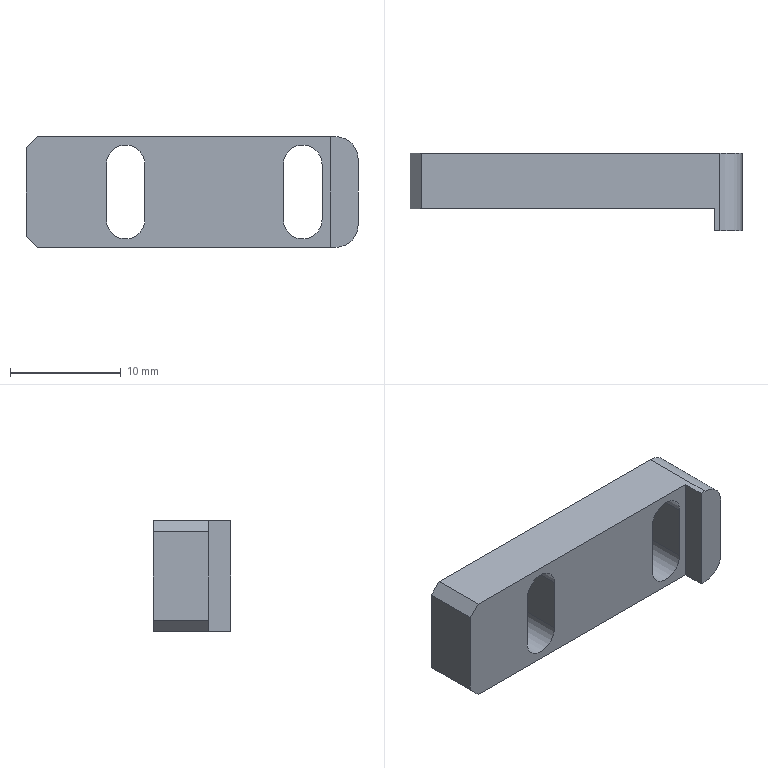Part | SolidWorks | features Chamfer 1, Extrusion 1, Fillet 1, ICE 1 | 1 solid | 20 faces | box 30 x 7 x 10 mm | volume 1262 mm3 | plane 14 | cylinder 6 | commonest cylinder face diameters 3.5 x4 4 x2
STEP:
#1=CARTESIAN_POINT('',(0.,-7.,3.));
#2=VERTEX_POINT('',#1);
#3=CARTESIAN_POINT('',(0.,-7.,-3.));
#4=VERTEX_POINT('',#3);
#5=CARTESIAN_POINT('',(0.,-7.,5.));
#6=DIRECTION('',(0.,0.,-1.));
#7=VECTOR('',#6,1000.);
#8=LINE('',#5,#7);
#9=EDGE_CURVE('',#2,#4,#8,.T.);
#10=ORIENTED_EDGE('',*,*,#9,.T.);
#11=CARTESIAN_POINT('',(0.,0.,-3.));
#12=VERTEX_POINT('',#11);
#13=CARTESIAN_POINT('',(0.,0.,-3.));
#14=DIRECTION('',(0.,1.,0.));
#15=VECTOR('',#14,1000.);
#16=LINE('',#13,#15);
#17=EDGE_CURVE('',#4,#12,#16,.T.);
#18=ORIENTED_EDGE('',*,*,#17,.T.);
#19=CARTESIAN_POINT('',(0.,0.,3.));
#20=VERTEX_POINT('',#19);
#21=CARTESIAN_POINT('',(0.,0.,5.));
#22=DIRECTION('',(0.,0.,-1.));
#23=VECTOR('',#22,1000.);
#24=LINE('',#21,#23);
#25=EDGE_CURVE('',#20,#12,#24,.T.);
#26=ORIENTED_EDGE('',*,*,#25,.F.);
#27=CARTESIAN_POINT('',(0.,0.,3.));
#28=DIRECTION('',(0.,-1.,0.));
#29=VECTOR('',#28,1000.);
#30=LINE('',#27,#29);
#31=EDGE_CURVE('',#20,#2,#30,.T.);
#32=ORIENTED_EDGE('',*,*,#31,.T.);
#33=EDGE_LOOP('',(#10,#18,#26,#32));
#34=FACE_OUTER_BOUND('',#33,.T.);
#35=CARTESIAN_POINT('',(0.,0.,5.));
#36=DIRECTION('',(-1.,0.,0.));
#37=DIRECTION('',(0.,-1.,0.));
#38=AXIS2_PLACEMENT_3D('',#35,#36,#37);
#39=PLANE('',#38);
#40=ADVANCED_FACE('',(#34),#39,.F.);
#41=CARTESIAN_POINT('',(-3.25,0.,-2.5));
#42=VERTEX_POINT('',#41);
#43=CARTESIAN_POINT('',(-3.25,0.,2.5));
#44=VERTEX_POINT('',#43);
#45=CARTESIAN_POINT('',(-3.25,0.,2.5));
#46=DIRECTION('',(0.,0.,1.));
#47=VECTOR('',#46,1000.);
#48=LINE('',#45,#47);
#49=EDGE_CURVE('',#42,#44,#48,.T.);
#50=ORIENTED_EDGE('',*,*,#49,.T.);
#51=CARTESIAN_POINT('',(-6.75,0.,2.5));
#52=VERTEX_POINT('',#51);
#53=CARTESIAN_POINT('',(-5.,0.,2.5));
#54=DIRECTION('',(0.,-1.,0.));
#55=DIRECTION('',(1.,0.,0.));
#56=AXIS2_PLACEMENT_3D('',#53,#54,#55);
#57=CIRCLE('',#56,1.75);
#58=EDGE_CURVE('',#44,#52,#57,.T.);
#59=ORIENTED_EDGE('',*,*,#58,.T.);
#60=CARTESIAN_POINT('',(-6.75,0.,-2.5));
#61=VERTEX_POINT('',#60);
#62=CARTESIAN_POINT('',(-6.75,0.,2.5));
#63=DIRECTION('',(0.,0.,-1.));
#64=VECTOR('',#63,1000.);
#65=LINE('',#62,#64);
#66=EDGE_CURVE('',#52,#61,#65,.T.);
#67=ORIENTED_EDGE('',*,*,#66,.T.);
#68=CARTESIAN_POINT('',(-5.,0.,-2.5));
#69=DIRECTION('',(0.,-1.,0.));
#70=DIRECTION('',(1.,0.,0.));
#71=AXIS2_PLACEMENT_3D('',#68,#69,#70);
#72=CIRCLE('',#71,1.75);
#73=EDGE_CURVE('',#61,#42,#72,.T.);
#74=ORIENTED_EDGE('',*,*,#73,.T.);
#75=EDGE_LOOP('',(#50,#59,#67,#74));
#76=FACE_BOUND('',#75,.T.);
#77=CARTESIAN_POINT('',(-19.25,0.,-2.5));
#78=VERTEX_POINT('',#77);
#79=CARTESIAN_POINT('',(-19.25,0.,2.5));
#80=VERTEX_POINT('',#79);
#81=CARTESIAN_POINT('',(-19.25,0.,2.5));
#82=DIRECTION('',(0.,0.,1.));
#83=VECTOR('',#82,1000.);
#84=LINE('',#81,#83);
#85=EDGE_CURVE('',#78,#80,#84,.T.);
#86=ORIENTED_EDGE('',*,*,#85,.T.);
#87=CARTESIAN_POINT('',(-22.75,0.,2.5));
#88=VERTEX_POINT('',#87);
#89=CARTESIAN_POINT('',(-21.,0.,2.5));
#90=DIRECTION('',(0.,-1.,0.));
#91=DIRECTION('',(1.,0.,0.));
#92=AXIS2_PLACEMENT_3D('',#89,#90,#91);
#93=CIRCLE('',#92,1.75);
#94=EDGE_CURVE('',#80,#88,#93,.T.);
#95=ORIENTED_EDGE('',*,*,#94,.T.);
#96=CARTESIAN_POINT('',(-22.75,0.,-2.5));
#97=VERTEX_POINT('',#96);
#98=CARTESIAN_POINT('',(-22.75,0.,2.5));
#99=DIRECTION('',(0.,0.,-1.));
#100=VECTOR('',#99,1000.);
#101=LINE('',#98,#100);
#102=EDGE_CURVE('',#88,#97,#101,.T.);
#103=ORIENTED_EDGE('',*,*,#102,.T.);
#104=CARTESIAN_POINT('',(-21.,0.,-2.5));
#105=DIRECTION('',(0.,-1.,0.));
#106=DIRECTION('',(1.,0.,0.));
#107=AXIS2_PLACEMENT_3D('',#104,#105,#106);
#108=CIRCLE('',#107,1.75);
#109=EDGE_CURVE('',#97,#78,#108,.T.);
#110=ORIENTED_EDGE('',*,*,#109,.T.);
#111=EDGE_LOOP('',(#86,#95,#103,#110));
#112=FACE_BOUND('',#111,.T.);
#113=CARTESIAN_POINT('',(-30.,0.,4.));
#114=VERTEX_POINT('',#113);
#115=CARTESIAN_POINT('',(-30.,0.,-4.));
#116=VERTEX_POINT('',#115);
#117=CARTESIAN_POINT('',(-30.,0.,5.));
#118=DIRECTION('',(0.,0.,-1.));
#119=VECTOR('',#118,1000.);
#120=LINE('',#117,#119);
#121=EDGE_CURVE('',#114,#116,#120,.T.);
#122=ORIENTED_EDGE('',*,*,#121,.F.);
#123=CARTESIAN_POINT('',(-29.,0.,5.));
#124=VERTEX_POINT('',#123);
#125=CARTESIAN_POINT('',(-29.,0.,5.));
#126=DIRECTION('',(0.7071,0.,0.7071));
#127=VECTOR('',#126,1000.);
#128=LINE('',#125,#127);
#129=EDGE_CURVE('',#114,#124,#128,.T.);
#130=ORIENTED_EDGE('',*,*,#129,.T.);
#131=CARTESIAN_POINT('',(-2.,0.,5.));
#132=VERTEX_POINT('',#131);
#133=CARTESIAN_POINT('',(0.,0.,5.));
#134=DIRECTION('',(-1.,0.,0.));
#135=VECTOR('',#134,1000.);
#136=LINE('',#133,#135);
#137=EDGE_CURVE('',#132,#124,#136,.T.);
#138=ORIENTED_EDGE('',*,*,#137,.F.);
#139=CARTESIAN_POINT('',(-2.,0.,3.));
#140=DIRECTION('',(0.,1.,0.));
#141=DIRECTION('',(1.,0.,0.));
#142=AXIS2_PLACEMENT_3D('',#139,#140,#141);
#143=CIRCLE('',#142,2.);
#144=EDGE_CURVE('',#132,#20,#143,.T.);
#145=ORIENTED_EDGE('',*,*,#144,.T.);
#146=ORIENTED_EDGE('',*,*,#25,.T.);
#147=CARTESIAN_POINT('',(-2.,0.,-5.));
#148=VERTEX_POINT('',#147);
#149=CARTESIAN_POINT('',(-2.,0.,-3.));
#150=DIRECTION('',(0.,1.,0.));
#151=DIRECTION('',(1.,0.,0.));
#152=AXIS2_PLACEMENT_3D('',#149,#150,#151);
#153=CIRCLE('',#152,2.);
#154=EDGE_CURVE('',#12,#148,#153,.T.);
#155=ORIENTED_EDGE('',*,*,#154,.T.);
#156=CARTESIAN_POINT('',(-29.,0.,-5.));
#157=VERTEX_POINT('',#156);
#158=CARTESIAN_POINT('',(0.,0.,-5.));
#159=DIRECTION('',(-1.,0.,0.));
#160=VECTOR('',#159,1000.);
#161=LINE('',#158,#160);
#162=EDGE_CURVE('',#148,#157,#161,.T.);
#163=ORIENTED_EDGE('',*,*,#162,.T.);
#164=CARTESIAN_POINT('',(-30.,0.,-4.));
#165=DIRECTION('',(-0.7071,0.,0.7071));
#166=VECTOR('',#165,1000.);
#167=LINE('',#164,#166);
#168=EDGE_CURVE('',#157,#116,#167,.T.);
#169=ORIENTED_EDGE('',*,*,#168,.T.);
#170=EDGE_LOOP('',(#122,#130,#138,#145,#146,#155,#163,#169));
#171=FACE_OUTER_BOUND('',#170,.T.);
#172=CARTESIAN_POINT('',(0.,0.,5.));
#173=DIRECTION('',(0.,-1.,0.));
#174=DIRECTION('',(1.,0.,0.));
#175=AXIS2_PLACEMENT_3D('',#172,#173,#174);
#176=PLANE('',#175);
#177=ADVANCED_FACE('',(#76,#112,#171),#176,.F.);
#178=CARTESIAN_POINT('',(-30.,-5.,4.));
#179=VERTEX_POINT('',#178);
#180=CARTESIAN_POINT('',(-30.,-5.,-4.));
#181=VERTEX_POINT('',#180);
#182=CARTESIAN_POINT('',(-30.,-5.,5.));
#183=DIRECTION('',(0.,0.,-1.));
#184=VECTOR('',#183,1000.);
#185=LINE('',#182,#184);
#186=EDGE_CURVE('',#179,#181,#185,.T.);
#187=ORIENTED_EDGE('',*,*,#186,.F.);
#188=CARTESIAN_POINT('',(-30.,0.,4.));
#189=DIRECTION('',(0.,1.,0.));
#190=VECTOR('',#189,1000.);
#191=LINE('',#188,#190);
#192=EDGE_CURVE('',#179,#114,#191,.T.);
#193=ORIENTED_EDGE('',*,*,#192,.T.);
#194=ORIENTED_EDGE('',*,*,#121,.T.);
#195=CARTESIAN_POINT('',(-30.,-5.,-4.));
#196=DIRECTION('',(0.,-1.,0.));
#197=VECTOR('',#196,1000.);
#198=LINE('',#195,#197);
#199=EDGE_CURVE('',#116,#181,#198,.T.);
#200=ORIENTED_EDGE('',*,*,#199,.T.);
#201=EDGE_LOOP('',(#187,#193,#194,#200));
#202=FACE_OUTER_BOUND('',#201,.T.);
#203=CARTESIAN_POINT('',(-30.,0.,5.));
#204=DIRECTION('',(1.,0.,0.));
#205=DIRECTION('',(0.,0.,-1.));
#206=AXIS2_PLACEMENT_3D('',#203,#204,#205);
#207=PLANE('',#206);
#208=ADVANCED_FACE('',(#202),#207,.F.);
#209=CARTESIAN_POINT('',(-6.75,-5.,2.5));
#210=VERTEX_POINT('',#209);
#211=CARTESIAN_POINT('',(-6.75,-5.,-2.5));
#212=VERTEX_POINT('',#211);
#213=CARTESIAN_POINT('',(-6.75,-5.,2.5));
#214=DIRECTION('',(0.,0.,-1.));
#215=VECTOR('',#214,1000.);
#216=LINE('',#213,#215);
#217=EDGE_CURVE('',#210,#212,#216,.T.);
#218=ORIENTED_EDGE('',*,*,#217,.F.);
#219=CARTESIAN_POINT('',(-3.25,-5.,2.5));
#220=VERTEX_POINT('',#219);
#221=CARTESIAN_POINT('',(-5.,-5.,2.5));
#222=DIRECTION('',(0.,-1.,0.));
#223=DIRECTION('',(1.,0.,0.));
#224=AXIS2_PLACEMENT_3D('',#221,#222,#223);
#225=CIRCLE('',#224,1.75);
#226=EDGE_CURVE('',#220,#210,#225,.T.);
#227=ORIENTED_EDGE('',*,*,#226,.F.);
#228=CARTESIAN_POINT('',(-3.25,-5.,-2.5));
#229=VERTEX_POINT('',#228);
#230=CARTESIAN_POINT('',(-3.25,-5.,2.5));
#231=DIRECTION('',(0.,0.,1.));
#232=VECTOR('',#231,1000.);
#233=LINE('',#230,#232);
#234=EDGE_CURVE('',#229,#220,#233,.T.);
#235=ORIENTED_EDGE('',*,*,#234,.F.);
#236=CARTESIAN_POINT('',(-5.,-5.,-2.5));
#237=DIRECTION('',(0.,-1.,0.));
#238=DIRECTION('',(1.,0.,0.));
#239=AXIS2_PLACEMENT_3D('',#236,#237,#238);
#240=CIRCLE('',#239,1.75);
#241=EDGE_CURVE('',#212,#229,#240,.T.);
#242=ORIENTED_EDGE('',*,*,#241,.F.);
#243=EDGE_LOOP('',(#218,#227,#235,#242));
#244=FACE_BOUND('',#243,.T.);
#245=CARTESIAN_POINT('',(-22.75,-5.,2.5));
#246=VERTEX_POINT('',#245);
#247=CARTESIAN_POINT('',(-22.75,-5.,-2.5));
#248=VERTEX_POINT('',#247);
#249=CARTESIAN_POINT('',(-22.75,-5.,2.5));
#250=DIRECTION('',(0.,0.,-1.));
#251=VECTOR('',#250,1000.);
#252=LINE('',#249,#251);
#253=EDGE_CURVE('',#246,#248,#252,.T.);
#254=ORIENTED_EDGE('',*,*,#253,.F.);
#255=CARTESIAN_POINT('',(-19.25,-5.,2.5));
#256=VERTEX_POINT('',#255);
#257=CARTESIAN_POINT('',(-21.,-5.,2.5));
#258=DIRECTION('',(0.,-1.,0.));
#259=DIRECTION('',(1.,0.,0.));
#260=AXIS2_PLACEMENT_3D('',#257,#258,#259);
#261=CIRCLE('',#260,1.75);
#262=EDGE_CURVE('',#256,#246,#261,.T.);
#263=ORIENTED_EDGE('',*,*,#262,.F.);
#264=CARTESIAN_POINT('',(-19.25,-5.,-2.5));
#265=VERTEX_POINT('',#264);
#266=CARTESIAN_POINT('',(-19.25,-5.,2.5));
#267=DIRECTION('',(0.,0.,1.));
#268=VECTOR('',#267,1000.);
#269=LINE('',#266,#268);
#270=EDGE_CURVE('',#265,#256,#269,.T.);
#271=ORIENTED_EDGE('',*,*,#270,.F.);
#272=CARTESIAN_POINT('',(-21.,-5.,-2.5));
#273=DIRECTION('',(0.,-1.,0.));
#274=DIRECTION('',(1.,0.,0.));
#275=AXIS2_PLACEMENT_3D('',#272,#273,#274);
#276=CIRCLE('',#275,1.75);
#277=EDGE_CURVE('',#248,#265,#276,.T.);
#278=ORIENTED_EDGE('',*,*,#277,.F.);
#279=EDGE_LOOP('',(#254,#263,#271,#278));
#280=FACE_BOUND('',#279,.T.);
#281=CARTESIAN_POINT('',(-29.,-5.,5.));
#282=VERTEX_POINT('',#281);
#283=CARTESIAN_POINT('',(-2.5,-5.,5.));
#284=VERTEX_POINT('',#283);
#285=CARTESIAN_POINT('',(-30.,-5.,5.));
#286=DIRECTION('',(1.,0.,0.));
#287=VECTOR('',#286,1000.);
#288=LINE('',#285,#287);
#289=EDGE_CURVE('',#282,#284,#288,.T.);
#290=ORIENTED_EDGE('',*,*,#289,.F.);
#291=CARTESIAN_POINT('',(-29.,-5.,5.));
#292=DIRECTION('',(-0.7071,0.,-0.7071));
#293=VECTOR('',#292,1000.);
#294=LINE('',#291,#293);
#295=EDGE_CURVE('',#282,#179,#294,.T.);
#296=ORIENTED_EDGE('',*,*,#295,.T.);
#297=ORIENTED_EDGE('',*,*,#186,.T.);
#298=CARTESIAN_POINT('',(-29.,-5.,-5.));
#299=VERTEX_POINT('',#298);
#300=CARTESIAN_POINT('',(-30.,-5.,-4.));
#301=DIRECTION('',(0.7071,0.,-0.7071));
#302=VECTOR('',#301,1000.);
#303=LINE('',#300,#302);
#304=EDGE_CURVE('',#181,#299,#303,.T.);
#305=ORIENTED_EDGE('',*,*,#304,.T.);
#306=CARTESIAN_POINT('',(-2.5,-5.,-5.));
#307=VERTEX_POINT('',#306);
#308=CARTESIAN_POINT('',(-30.,-5.,-5.));
#309=DIRECTION('',(1.,0.,0.));
#310=VECTOR('',#309,1000.);
#311=LINE('',#308,#310);
#312=EDGE_CURVE('',#299,#307,#311,.T.);
#313=ORIENTED_EDGE('',*,*,#312,.T.);
#314=CARTESIAN_POINT('',(-2.5,-5.,5.));
#315=DIRECTION('',(0.,0.,-1.));
#316=VECTOR('',#315,1000.);
#317=LINE('',#314,#316);
#318=EDGE_CURVE('',#284,#307,#317,.T.);
#319=ORIENTED_EDGE('',*,*,#318,.F.);
#320=EDGE_LOOP('',(#290,#296,#297,#305,#313,#319));
#321=FACE_OUTER_BOUND('',#320,.T.);
#322=CARTESIAN_POINT('',(-30.,-5.,5.));
#323=DIRECTION('',(0.,1.,0.));
#324=DIRECTION('',(-1.,0.,0.));
#325=AXIS2_PLACEMENT_3D('',#322,#323,#324);
#326=PLANE('',#325);
#327=ADVANCED_FACE('',(#244,#280,#321),#326,.F.);
#328=CARTESIAN_POINT('',(-2.5,-7.,-5.));
#329=VERTEX_POINT('',#328);
#330=CARTESIAN_POINT('',(-2.5,-7.,-5.));
#331=DIRECTION('',(0.,-1.,0.));
#332=VECTOR('',#331,1000.);
#333=LINE('',#330,#332);
#334=EDGE_CURVE('',#307,#329,#333,.T.);
#335=ORIENTED_EDGE('',*,*,#334,.T.);
#336=CARTESIAN_POINT('',(-2.5,-7.,5.));
#337=VERTEX_POINT('',#336);
#338=CARTESIAN_POINT('',(-2.5,-7.,5.));
#339=DIRECTION('',(0.,0.,-1.));
#340=VECTOR('',#339,1000.);
#341=LINE('',#338,#340);
#342=EDGE_CURVE('',#337,#329,#341,.T.);
#343=ORIENTED_EDGE('',*,*,#342,.F.);
#344=CARTESIAN_POINT('',(-2.5,-7.,5.));
#345=DIRECTION('',(0.,-1.,0.));
#346=VECTOR('',#345,1000.);
#347=LINE('',#344,#346);
#348=EDGE_CURVE('',#284,#337,#347,.T.);
#349=ORIENTED_EDGE('',*,*,#348,.F.);
#350=ORIENTED_EDGE('',*,*,#318,.T.);
#351=EDGE_LOOP('',(#335,#343,#349,#350));
#352=FACE_OUTER_BOUND('',#351,.T.);
#353=CARTESIAN_POINT('',(-2.5,-7.,5.));
#354=DIRECTION('',(1.,0.,0.));
#355=DIRECTION('',(0.,1.,0.));
#356=AXIS2_PLACEMENT_3D('',#353,#354,#355);
#357=PLANE('',#356);
#358=ADVANCED_FACE('',(#352),#357,.F.);
#359=CARTESIAN_POINT('',(-2.,-7.,-5.));
#360=VERTEX_POINT('',#359);
#361=CARTESIAN_POINT('',(0.,-7.,-5.));
#362=DIRECTION('',(1.,0.,0.));
#363=VECTOR('',#362,1000.);
#364=LINE('',#361,#363);
#365=EDGE_CURVE('',#329,#360,#364,.T.);
#366=ORIENTED_EDGE('',*,*,#365,.T.);
#367=CARTESIAN_POINT('',(-2.,-7.,-3.));
#368=DIRECTION('',(0.,-1.,0.));
#369=DIRECTION('',(0.,0.,1.));
#370=AXIS2_PLACEMENT_3D('',#367,#368,#369);
#371=CIRCLE('',#370,2.);
#372=EDGE_CURVE('',#360,#4,#371,.T.);
#373=ORIENTED_EDGE('',*,*,#372,.T.);
#374=ORIENTED_EDGE('',*,*,#9,.F.);
#375=CARTESIAN_POINT('',(-2.,-7.,5.));
#376=VERTEX_POINT('',#375);
#377=CARTESIAN_POINT('',(-2.,-7.,3.));
#378=DIRECTION('',(0.,-1.,0.));
#379=DIRECTION('',(0.,0.,1.));
#380=AXIS2_PLACEMENT_3D('',#377,#378,#379);
#381=CIRCLE('',#380,2.);
#382=EDGE_CURVE('',#2,#376,#381,.T.);
#383=ORIENTED_EDGE('',*,*,#382,.T.);
#384=CARTESIAN_POINT('',(0.,-7.,5.));
#385=DIRECTION('',(1.,0.,0.));
#386=VECTOR('',#385,1000.);
#387=LINE('',#384,#386);
#388=EDGE_CURVE('',#337,#376,#387,.T.);
#389=ORIENTED_EDGE('',*,*,#388,.F.);
#390=ORIENTED_EDGE('',*,*,#342,.T.);
#391=EDGE_LOOP('',(#366,#373,#374,#383,#389,#390));
#392=FACE_OUTER_BOUND('',#391,.T.);
#393=CARTESIAN_POINT('',(0.,-7.,5.));
#394=DIRECTION('',(0.,1.,0.));
#395=DIRECTION('',(0.,0.,1.));
#396=AXIS2_PLACEMENT_3D('',#393,#394,#395);
#397=PLANE('',#396);
#398=ADVANCED_FACE('',(#392),#397,.F.);
#399=ORIENTED_EDGE('',*,*,#137,.T.);
#400=CARTESIAN_POINT('',(-29.,-7.,5.));
#401=DIRECTION('',(0.,-1.,0.));
#402=VECTOR('',#401,1000.);
#403=LINE('',#400,#402);
#404=EDGE_CURVE('',#124,#282,#403,.T.);
#405=ORIENTED_EDGE('',*,*,#404,.T.);
#406=ORIENTED_EDGE('',*,*,#289,.T.);
#407=ORIENTED_EDGE('',*,*,#348,.T.);
#408=ORIENTED_EDGE('',*,*,#388,.T.);
#409=CARTESIAN_POINT('',(-2.,-7.,5.));
#410=DIRECTION('',(0.,1.,0.));
#411=VECTOR('',#410,1000.);
#412=LINE('',#409,#411);
#413=EDGE_CURVE('',#376,#132,#412,.T.);
#414=ORIENTED_EDGE('',*,*,#413,.T.);
#415=EDGE_LOOP('',(#399,#405,#406,#407,#408,#414));
#416=FACE_OUTER_BOUND('',#415,.T.);
#417=CARTESIAN_POINT('',(0.,-7.,5.));
#418=DIRECTION('',(0.,0.,-1.));
#419=DIRECTION('',(-1.,0.,0.));
#420=AXIS2_PLACEMENT_3D('',#417,#418,#419);
#421=PLANE('',#420);
#422=ADVANCED_FACE('',(#416),#421,.F.);
#423=ORIENTED_EDGE('',*,*,#312,.F.);
#424=CARTESIAN_POINT('',(-29.,0.,-5.));
#425=DIRECTION('',(0.,1.,0.));
#426=VECTOR('',#425,1000.);
#427=LINE('',#424,#426);
#428=EDGE_CURVE('',#299,#157,#427,.T.);
#429=ORIENTED_EDGE('',*,*,#428,.T.);
#430=ORIENTED_EDGE('',*,*,#162,.F.);
#431=CARTESIAN_POINT('',(-2.,-7.,-5.));
#432=DIRECTION('',(0.,-1.,0.));
#433=VECTOR('',#432,1000.);
#434=LINE('',#431,#433);
#435=EDGE_CURVE('',#148,#360,#434,.T.);
#436=ORIENTED_EDGE('',*,*,#435,.T.);
#437=ORIENTED_EDGE('',*,*,#365,.F.);
#438=ORIENTED_EDGE('',*,*,#334,.F.);
#439=EDGE_LOOP('',(#423,#429,#430,#436,#437,#438));
#440=FACE_OUTER_BOUND('',#439,.T.);
#441=CARTESIAN_POINT('',(0.,-7.,-5.));
#442=DIRECTION('',(0.,0.,-1.));
#443=DIRECTION('',(-1.,0.,0.));
#444=AXIS2_PLACEMENT_3D('',#441,#442,#443);
#445=PLANE('',#444);
#446=ADVANCED_FACE('',(#440),#445,.T.);
#447=ORIENTED_EDGE('',*,*,#262,.T.);
#448=CARTESIAN_POINT('',(-22.75,0.,2.5));
#449=DIRECTION('',(0.,-1.,0.));
#450=VECTOR('',#449,1000.);
#451=LINE('',#448,#450);
#452=EDGE_CURVE('',#88,#246,#451,.T.);
#453=ORIENTED_EDGE('',*,*,#452,.F.);
#454=ORIENTED_EDGE('',*,*,#94,.F.);
#455=CARTESIAN_POINT('',(-19.25,0.,2.5));
#456=DIRECTION('',(0.,-1.,0.));
#457=VECTOR('',#456,1000.);
#458=LINE('',#455,#457);
#459=EDGE_CURVE('',#80,#256,#458,.T.);
#460=ORIENTED_EDGE('',*,*,#459,.T.);
#461=EDGE_LOOP('',(#447,#453,#454,#460));
#462=FACE_OUTER_BOUND('',#461,.T.);
#463=CARTESIAN_POINT('',(-21.,0.,2.5));
#464=DIRECTION('',(0.,-1.,0.));
#465=DIRECTION('',(1.,0.,0.));
#466=AXIS2_PLACEMENT_3D('',#463,#464,#465);
#467=CYLINDRICAL_SURFACE('',#466,1.75);
#468=ADVANCED_FACE('',(#462),#467,.F.);
#469=ORIENTED_EDGE('',*,*,#270,.T.);
#470=ORIENTED_EDGE('',*,*,#459,.F.);
#471=ORIENTED_EDGE('',*,*,#85,.F.);
#472=CARTESIAN_POINT('',(-19.25,0.,-2.5));
#473=DIRECTION('',(0.,-1.,0.));
#474=VECTOR('',#473,1000.);
#475=LINE('',#472,#474);
#476=EDGE_CURVE('',#78,#265,#475,.T.);
#477=ORIENTED_EDGE('',*,*,#476,.T.);
#478=EDGE_LOOP('',(#469,#470,#471,#477));
#479=FACE_OUTER_BOUND('',#478,.T.);
#480=CARTESIAN_POINT('',(-19.25,0.,2.5));
#481=DIRECTION('',(1.,0.,0.));
#482=DIRECTION('',(0.,1.,0.));
#483=AXIS2_PLACEMENT_3D('',#480,#481,#482);
#484=PLANE('',#483);
#485=ADVANCED_FACE('',(#479),#484,.F.);
#486=ORIENTED_EDGE('',*,*,#277,.T.);
#487=ORIENTED_EDGE('',*,*,#476,.F.);
#488=ORIENTED_EDGE('',*,*,#109,.F.);
#489=CARTESIAN_POINT('',(-22.75,0.,-2.5));
#490=DIRECTION('',(0.,-1.,0.));
#491=VECTOR('',#490,1000.);
#492=LINE('',#489,#491);
#493=EDGE_CURVE('',#97,#248,#492,.T.);
#494=ORIENTED_EDGE('',*,*,#493,.T.);
#495=EDGE_LOOP('',(#486,#487,#488,#494));
#496=FACE_OUTER_BOUND('',#495,.T.);
#497=CARTESIAN_POINT('',(-21.,0.,-2.5));
#498=DIRECTION('',(0.,-1.,0.));
#499=DIRECTION('',(1.,0.,0.));
#500=AXIS2_PLACEMENT_3D('',#497,#498,#499);
#501=CYLINDRICAL_SURFACE('',#500,1.75);
#502=ADVANCED_FACE('',(#496),#501,.F.);
#503=ORIENTED_EDGE('',*,*,#253,.T.);
#504=ORIENTED_EDGE('',*,*,#493,.F.);
#505=ORIENTED_EDGE('',*,*,#102,.F.);
#506=ORIENTED_EDGE('',*,*,#452,.T.);
#507=EDGE_LOOP('',(#503,#504,#505,#506));
#508=FACE_OUTER_BOUND('',#507,.T.);
#509=CARTESIAN_POINT('',(-22.75,0.,2.5));
#510=DIRECTION('',(-1.,0.,0.));
#511=DIRECTION('',(0.,0.,1.));
#512=AXIS2_PLACEMENT_3D('',#509,#510,#511);
#513=PLANE('',#512);
#514=ADVANCED_FACE('',(#508),#513,.F.);
#515=ORIENTED_EDGE('',*,*,#226,.T.);
#516=CARTESIAN_POINT('',(-6.75,0.,2.5));
#517=DIRECTION('',(0.,-1.,0.));
#518=VECTOR('',#517,1000.);
#519=LINE('',#516,#518);
#520=EDGE_CURVE('',#52,#210,#519,.T.);
#521=ORIENTED_EDGE('',*,*,#520,.F.);
#522=ORIENTED_EDGE('',*,*,#58,.F.);
#523=CARTESIAN_POINT('',(-3.25,0.,2.5));
#524=DIRECTION('',(0.,-1.,0.));
#525=VECTOR('',#524,1000.);
#526=LINE('',#523,#525);
#527=EDGE_CURVE('',#44,#220,#526,.T.);
#528=ORIENTED_EDGE('',*,*,#527,.T.);
#529=EDGE_LOOP('',(#515,#521,#522,#528));
#530=FACE_OUTER_BOUND('',#529,.T.);
#531=CARTESIAN_POINT('',(-5.,0.,2.5));
#532=DIRECTION('',(0.,-1.,0.));
#533=DIRECTION('',(1.,0.,0.));
#534=AXIS2_PLACEMENT_3D('',#531,#532,#533);
#535=CYLINDRICAL_SURFACE('',#534,1.75);
#536=ADVANCED_FACE('',(#530),#535,.F.);
#537=ORIENTED_EDGE('',*,*,#234,.T.);
#538=ORIENTED_EDGE('',*,*,#527,.F.);
#539=ORIENTED_EDGE('',*,*,#49,.F.);
#540=CARTESIAN_POINT('',(-3.25,0.,-2.5));
#541=DIRECTION('',(0.,-1.,0.));
#542=VECTOR('',#541,1000.);
#543=LINE('',#540,#542);
#544=EDGE_CURVE('',#42,#229,#543,.T.);
#545=ORIENTED_EDGE('',*,*,#544,.T.);
#546=EDGE_LOOP('',(#537,#538,#539,#545));
#547=FACE_OUTER_BOUND('',#546,.T.);
#548=CARTESIAN_POINT('',(-3.25,0.,2.5));
#549=DIRECTION('',(1.,0.,0.));
#550=DIRECTION('',(0.,1.,0.));
#551=AXIS2_PLACEMENT_3D('',#548,#549,#550);
#552=PLANE('',#551);
#553=ADVANCED_FACE('',(#547),#552,.F.);
#554=ORIENTED_EDGE('',*,*,#241,.T.);
#555=ORIENTED_EDGE('',*,*,#544,.F.);
#556=ORIENTED_EDGE('',*,*,#73,.F.);
#557=CARTESIAN_POINT('',(-6.75,0.,-2.5));
#558=DIRECTION('',(0.,-1.,0.));
#559=VECTOR('',#558,1000.);
#560=LINE('',#557,#559);
#561=EDGE_CURVE('',#61,#212,#560,.T.);
#562=ORIENTED_EDGE('',*,*,#561,.T.);
#563=EDGE_LOOP('',(#554,#555,#556,#562));
#564=FACE_OUTER_BOUND('',#563,.T.);
#565=CARTESIAN_POINT('',(-5.,0.,-2.5));
#566=DIRECTION('',(0.,-1.,0.));
#567=DIRECTION('',(1.,0.,0.));
#568=AXIS2_PLACEMENT_3D('',#565,#566,#567);
#569=CYLINDRICAL_SURFACE('',#568,1.75);
#570=ADVANCED_FACE('',(#564),#569,.F.);
#571=ORIENTED_EDGE('',*,*,#217,.T.);
#572=ORIENTED_EDGE('',*,*,#561,.F.);
#573=ORIENTED_EDGE('',*,*,#66,.F.);
#574=ORIENTED_EDGE('',*,*,#520,.T.);
#575=EDGE_LOOP('',(#571,#572,#573,#574));
#576=FACE_OUTER_BOUND('',#575,.T.);
#577=CARTESIAN_POINT('',(-6.75,0.,2.5));
#578=DIRECTION('',(-1.,0.,0.));
#579=DIRECTION('',(0.,-1.,0.));
#580=AXIS2_PLACEMENT_3D('',#577,#578,#579);
#581=PLANE('',#580);
#582=ADVANCED_FACE('',(#576),#581,.F.);
#583=ORIENTED_EDGE('',*,*,#372,.F.);
#584=ORIENTED_EDGE('',*,*,#435,.F.);
#585=ORIENTED_EDGE('',*,*,#154,.F.);
#586=ORIENTED_EDGE('',*,*,#17,.F.);
#587=EDGE_LOOP('',(#583,#584,#585,#586));
#588=FACE_OUTER_BOUND('',#587,.T.);
#589=CARTESIAN_POINT('',(-2.,0.,-3.));
#590=DIRECTION('',(0.,-1.,0.));
#591=DIRECTION('',(1.,0.,0.));
#592=AXIS2_PLACEMENT_3D('',#589,#590,#591);
#593=CYLINDRICAL_SURFACE('',#592,2.);
#594=ADVANCED_FACE('',(#588),#593,.T.);
#595=ORIENTED_EDGE('',*,*,#382,.F.);
#596=ORIENTED_EDGE('',*,*,#31,.F.);
#597=ORIENTED_EDGE('',*,*,#144,.F.);
#598=ORIENTED_EDGE('',*,*,#413,.F.);
#599=EDGE_LOOP('',(#595,#596,#597,#598));
#600=FACE_OUTER_BOUND('',#599,.T.);
#601=CARTESIAN_POINT('',(-2.,-7.,3.));
#602=DIRECTION('',(0.,1.,0.));
#603=DIRECTION('',(-1.,0.,0.));
#604=AXIS2_PLACEMENT_3D('',#601,#602,#603);
#605=CYLINDRICAL_SURFACE('',#604,2.);
#606=ADVANCED_FACE('',(#600),#605,.T.);
#607=ORIENTED_EDGE('',*,*,#129,.F.);
#608=ORIENTED_EDGE('',*,*,#192,.F.);
#609=ORIENTED_EDGE('',*,*,#295,.F.);
#610=ORIENTED_EDGE('',*,*,#404,.F.);
#611=EDGE_LOOP('',(#607,#608,#609,#610));
#612=FACE_OUTER_BOUND('',#611,.T.);
#613=CARTESIAN_POINT('',(-29.,-7.,5.));
#614=DIRECTION('',(0.7071,0.,-0.7071));
#615=DIRECTION('',(0.,-1.,0.));
#616=AXIS2_PLACEMENT_3D('',#613,#614,#615);
#617=PLANE('',#616);
#618=ADVANCED_FACE('',(#612),#617,.F.);
#619=ORIENTED_EDGE('',*,*,#168,.F.);
#620=ORIENTED_EDGE('',*,*,#428,.F.);
#621=ORIENTED_EDGE('',*,*,#304,.F.);
#622=ORIENTED_EDGE('',*,*,#199,.F.);
#623=EDGE_LOOP('',(#619,#620,#621,#622));
#624=FACE_OUTER_BOUND('',#623,.T.);
#625=CARTESIAN_POINT('',(-30.,0.,-4.));
#626=DIRECTION('',(-0.7071,0.,-0.7071));
#627=DIRECTION('',(0.,1.,0.));
#628=AXIS2_PLACEMENT_3D('',#625,#626,#627);
#629=PLANE('',#628);
#630=ADVANCED_FACE('',(#624),#629,.T.);
#631=CLOSED_SHELL('',(#40,#177,#208,#327,#358,#398,#422,#446,#468,#485,#502,#514,#536,#553,#570,#582,#594,#606,#618,#630));
#632=MANIFOLD_SOLID_BREP('',#631);
#633=CARTESIAN_POINT('',(0.,0.,0.));
#634=DIRECTION('',(0.,0.,1.));
#635=DIRECTION('',(1.,0.,0.));
#636=AXIS2_PLACEMENT_3D('',#633,#634,#635);
#637=(LENGTH_UNIT()NAMED_UNIT(*)SI_UNIT(.MILLI.,.METRE.));
#638=UNCERTAINTY_MEASURE_WITH_UNIT(LENGTH_MEASURE(0.00001),#637,'','');
#639=(NAMED_UNIT(*)PLANE_ANGLE_UNIT()SI_UNIT($,.RADIAN.));
#640=(NAMED_UNIT(*)SI_UNIT($,.STERADIAN.)SOLID_ANGLE_UNIT());
#641=(GEOMETRIC_REPRESENTATION_CONTEXT(3)GLOBAL_UNCERTAINTY_ASSIGNED_CONTEXT((#638))GLOBAL_UNIT_ASSIGNED_CONTEXT((#637,#639,#640))REPRESENTATION_CONTEXT('',''));
#642=ADVANCED_BREP_SHAPE_REPRESENTATION('',(#632,#636),#641);